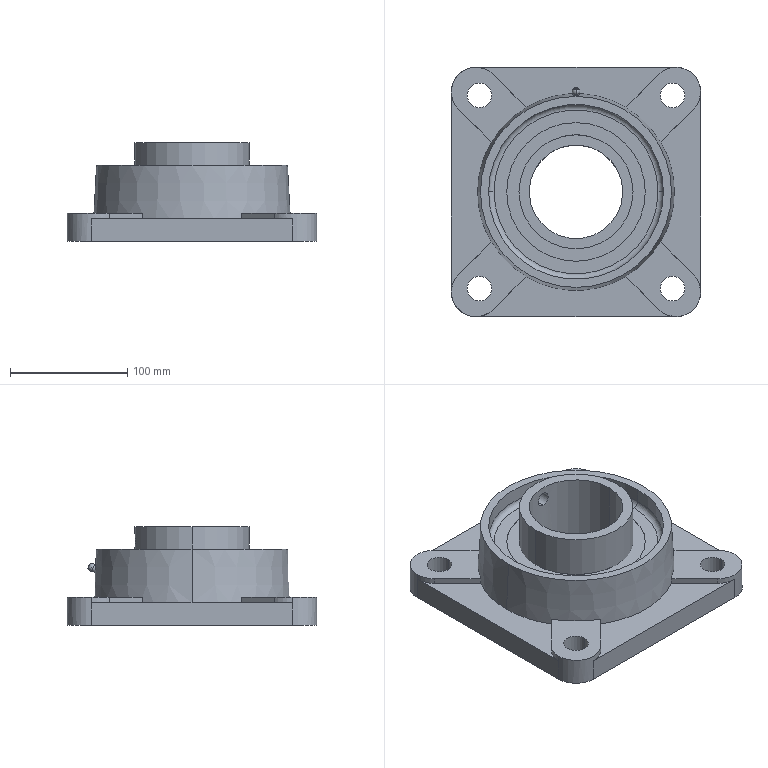Part | SolidWorks | features Revolution 5, Boss 2, RevCut 2, CirPattern 1, Cut 1, Extrusion 1, RefAxis 1 | 18 solids | 148 faces | box 213 x 213 x 84.3 mm | volume 1088893 mm3 | cylinder 58 | plane 38 | sphere 38 | torus 12 | cone 2 | commonest cylinder face diameters 42 x12 6 x10 21 x8 118.4 x8 96.4 x4 97.4 x4